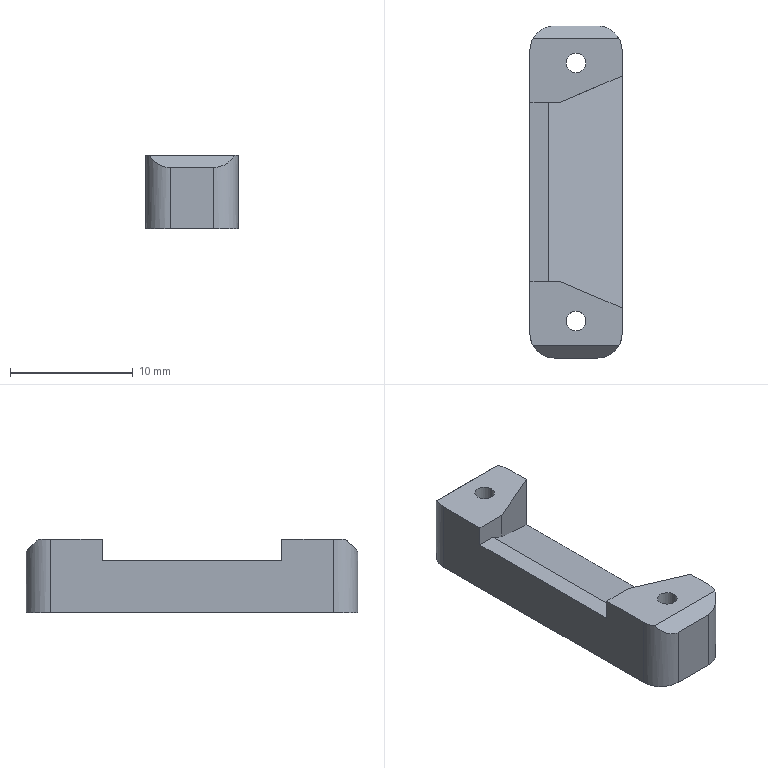NC program | NX | posted with a generic post | part box 7.5 x 27 x 6 mm
Whole program:
N10 G17 G21 G94 G90
(FLOOR_FACING , TOOL : D4-ROUGH)
N12 T01 M6
N14 G54
N16 G17 G0 G90 X20.5 Y-6. B0. C0. S4500 M3
N18 G43 Z30. H1
N20 Z2.05
N22 G94 G1 Z0.05 F800.
N24 X18.5
N26 X-25.5
N28 Y-3.15
N30 X18.5
N32 Y-0.3
N34 X-25.5
N36 Y2.55
N38 X18.5
N40 Y5.4
N42 X-25.5
N44 X-27.5
N46 Z2.05
N48 G0 Z30.
(ADAPTIVE_MILLING , TOOL : D4-ROUGH)
N50 X12.644 Y-13.007 S6500
N52 Z-4.
N54 G1 X12.632 Y-12.858 Z-4.937 F3000.
N56 X12.62 Y-12.708 Z-5.308
N58 X12.609 Y-12.558 Z-5.58
N60 X12.597 Y-12.409 Z-5.8
N62 X12.586 Y-12.259 Z-5.984
N64 X12.574 Y-12.11 Z-6.142
N66 X12.562 Y-11.96 Z-6.28
N68 X12.551 Y-11.811 Z-6.4
N70 X12.539 Y-11.661 Z-6.505
N72 X12.528 Y-11.512 Z-6.598
N74 X12.516 Y-11.362 Z-6.679
N76 X12.504 Y-11.212 Z-6.75
N78 X12.493 Y-11.063 Z-6.81
N80 X12.481 Y-10.913 Z-6.862
N82 X12.469 Y-10.764 Z-6.905
N84 X12.458 Y-10.614 Z-6.939
N86 X12.446 Y-10.465 Z-6.966
N88 X12.435 Y-10.315 Z-6.985
N90 X12.423 Y-10.166 Z-6.996
N92 X12.411 Y-10.016 Z-7.
N94 X12.385 Y-9.631
N96 X12.343 Y-9.248
N98 G3 X12.139 Y-9. R0.411
N100 X10.441 Y-8.678 R4.8
N102 X4.61 Y-8.6 R119.19
N104 G1 X-22.42 Y-8.595
N106 G2 X-24.273 Y-7.318 R2.392
N108 X-24.996 Y-4.583 R6.41
N110 X-25.098 Y0.305 R72.272
N112 G1 X-25.084 Y6.056
N114 G2 X-23.686 Y7.858 R2.494
N116 X-21.022 Y8.504 R6.789
N118 X-14.784 Y8.6 R101.69
N120 G1 X15.404 Y8.599
N122 G2 X17.251 Y7.371 R2.358
N124 X17.976 Y4.794 R6.037
N126 X18.096 Y0.027 R59.589
N128 X18.08 Y-6.087 R351.529
N130 X16.659 Y-7.873 R2.516
N132 X13.962 Y-8.508 R6.951
N134 X11.484 Y-8.375 R13.968
N136 G3 X5.808 Y-8.202 R66.934
N138 G1 X3.17 Y-8.2
N140 X-21.22 Y-8.196
N142 G2 X-23.83 Y-6.438 R3.102
N144 X-24.577 Y-3.491 R7.626
N146 X-24.697 Y1.456 R66.876
N148 X-24.67 Y5.035 R58.858
N150 X-22.813 Y7.399 R3.188
N152 X-19.762 Y8.098 R8.244
N154 X-12.864 Y8.2 R115.56
N156 G1 X14.204
N158 G2 X16.795 Y6.508 R3.064
N160 X17.574 Y3.508 R7.495
N162 X17.696 Y-1.65 R69.612
N164 X17.67 Y-5.036 R56.842
N166 X15.82 Y-7.396 R3.181
N168 X12.634 Y-7.984 R6.699
N170 G3 X2.45 Y-7.8 R183.554
N172 G1 X-20.14 Y-7.797
N174 G2 X-23.411 Y-5.696 R3.573
N176 X-24.178 Y-2.476 R8.723
N178 X-24.276 Y4.061 R79.928
N180 X-22.101 Y6.961 R3.606
N182 X-18.807 Y7.693 R9.218
N184 X-12.119 Y7.8 R111.311
N186 G1 X13.191 Y7.799
N188 G2 X16.394 Y5.733 R3.555
N190 X17.17 Y2.545 R8.578
N192 X17.27 Y-4.111 R75.06
N194 X14.894 Y-7.032 R3.582
N196 X11.737 Y-7.494 R8.667
N198 G3 X3.2 Y-7.4 R494.474
N200 G1 X-19.3 Y-7.396
N202 G2 X-23.052 Y-4.918 R3.966
N204 X-23.786 Y-1.504 R10.045
N206 X-23.855 Y3.413 R41.458
N208 X-21.509 Y6.512 R3.917
N210 X-18.161 Y7.275 R9.576
N212 X-11.653 Y7.4 R95.247
N214 G1 X12.074
N216 G2 X16.057 Y4.907 R3.995
N218 X16.789 Y1.431 R10.225
N220 X16.859 Y-3.366 R45.312
N222 X14.249 Y-6.556 R3.798
N224 X11.089 Y-7.037 R9.799
N226 G1 X1.91 Y-7.
N228 X-18.34 Y-6.997
N230 G2 X-21.223 Y-6.167 R4.515
N232 X-22.992 Y-3.299 R5.233
N234 X-23.454 Y0.715 R17.702
N236 X-23.382 Y3.109 R11.55
N238 X-20.878 Y6.107 R4.192
N240 X-17.438 Y6.871 R10.238
N242 X-10.781 Y6.999 R97.585
N244 G1 X11.204 Y7.
N246 G2 X13.836 Y6.43 R4.91
N248 X15.896 Y3.622 R4.843
N250 X16.44 Y-0.349 R15.281
N252 X16.403 Y-2.985 R14.999
N254 X13.826 Y-6.02 R3.954
N256 X10.44 Y-6.596 R10.143
N258 X1.1 Y-6.6 R586.341
N260 G1 X-17.55 Y-6.597
N262 G2 X-20.222 Y-6.046 R5.358
N264 X-22.425 Y-3.215 R4.925
N266 X-23.027 Y0.747 R14.496
N268 X-22.721 Y3.317 R5.972
N270 X-20.014 Y5.814 R4.614
N272 X-16.342 Y6.497 R12.221
N274 X-8.304 Y6.6 R157.367
N276 G1 X10.604 Y6.598
N278 G2 X13.321 Y5.992 R5.18
N280 X15.47 Y3.078 R5.03
N282 X16.036 Y-1.101 R15.78
N284 X15.417 Y-3.866 R4.67
N286 X12.628 Y-5.776 R4.734
N288 X8.972 Y-6.193 R14.778
N290 G1 X7.232 Y-6.208
N292 X-10.456 Y-6.204
N294 G2 X-17.609 Y-6.175 R433.58
N296 X-21.802 Y-3.212 R4.627
N298 X-22.523 Y1.849 R11.022
N300 X-19.878 Y5.221 R4.433
N302 X-16.182 Y6.059 R10.727
N304 X-9.99 Y6.198 R88.623
N306 G1 X9.79 Y6.2
N308 G2 X12.327 Y5.809 R6.448
N310 X14.294 Y4.819 R4.458
N312 X15.561 Y2.607 R4.476
N314 G1 X15.65 Y1.749
N316 Y-1.751
N318 X15.546 Y-2.673
N320 X15.239 Y-3.551
N322 X14.745 Y-4.337
N324 X14.087 Y-4.995
N326 X13.301 Y-5.489
N328 X12.423 Y-5.796
N330 X11.5 Y-5.9
N332 X-11.501
N334 G3 X-16.303 Y-5.797 R64.238
N336 G2 X-19.105 Y-5.259 R6.166
N338 X-21.567 Y-2.233 R5.158
N340 X-22.028 Y1.428 R8.25
N342 X-19.401 Y4.778 R4.46
N344 X-15.681 Y5.647 R10.697
N346 X-12.415 Y5.785 R72.636
N348 X-11.499 Y5.9 R3.787
N350 G1 X11.501
N352 G2 X12.347 Y5.803 R7.502
N354 G3 X12.82 Y6.348 R0.4
N356 X12.567 Y6.59 Z-6.955 R0.548
N358 G1 X12.204 Y6.819 Z-6.9
N360 X11.738 Y7.108 F15000.
N362 X11.657 Y7.132
N364 X11.574 Y7.143
N366 X-11.641 Y7.125
N368 G3 X-12.018 Y6.86 R0.401
N370 G1 X-12.076 Y6.51 Z-6.945 F3000.
N372 X-12.118 Y6.158 Z-6.99
N374 X-12.13 Y6.082 Z-7.
N376 G2 X-12.415 Y5.785 R0.402
N378 X-14.107 Y5.528 R8.134
N380 G3 X-17.929 Y5.004 R19.887
N382 X-20.854 Y3.172 R5.32
N384 X-21.679 Y-0.221 R4.872
N386 X-20.236 Y-3.903 R6.311
N388 X-17.026 Y-5.43 R4.937
N390 X-13.014 Y-5.593 R52.658
N392 X-11.738 Y-5.873 R3.505
N394 G2 X-12.984 Y-5.6 R3.404
N396 G3 X-15.088 Y-5.2 R7.056
N398 G2 X-17.861 Y-4.754 R11.202
N400 X-20.896 Y-1.405 R4.893
N402 X-20.726 Y2.106 R4.789
N404 X-17.971 Y4.394 R4.824
N406 X-14.715 Y5.048 R13.604
N408 G3 X-13.797 Y5.187 R3.561
N410 G2 X-12.705 Y5.706 R3.586
N412 G3 X-13.921 Y5.112 R3.961
N414 G2 X-15.964 Y4.648 R12.273
N416 G3 X-19.001 Y3.502 R7.713
N418 X-20.662 Y-0.761 R4.201
N420 X-17.01 Y-4.615 R4.682
N422 X-14.238 Y-5.062 R33.87
N424 G1 X-13.819 Y-5.163
N426 X-13.301 Y-5.489
N428 G3 X-14.702 Y-4.76 R4.998
N430 G2 X-17.049 Y-4.13 R32.062
N432 X-20.048 Y0.515 R4.386
N434 X-17.922 Y3.389 R3.99
N436 X-15.133 Y4.358 R11.169
N438 G3 X-14.494 Y4.595 R1.572
N440 G2 X-13.811 Y5.174 R2.943
N442 G3 X-14.619 Y4.48 R4.496
N444 G2 X-16.301 Y3.804 R9.75
N446 G3 X-18.77 Y2.262 R5.667
N448 X-18.251 Y-2.958 R3.708
N450 X-15.823 Y-4.171 R6.478
N452 G2 X-14.434 Y-4.652 R8.607
N454 G1 X-14.062 Y-5.011
N456 G3 X-15.558 Y-3.954 R3.954
N458 G2 X-17.711 Y-2.685 R7.477
N460 X-17.68 Y2.264 R3.248
N462 X-15.497 Y3.592 R8.764
N464 G3 X-14.868 Y4.175 R0.994
N466 G1 X-14.528 Y4.556
N468 G3 X-15.073 Y3.819 R2.508
N470 G2 X-16.347 Y2.914 R6.844
N472 G3 X-18.093 Y1.023 R4.263
N474 X-17.232 Y-2.462 R3.178
N476 X-15.333 Y-3.76 R9.128
N478 G2 X-14.745 Y-4.337 R1.154
N480 G1 X-14.554 Y-4.528
N482 G2 X-15.056 Y-3.851 R2.83
N484 G3 X-16.37 Y-2.657 R17.482
N486 G2 X-17.465 Y-0.223 R3.065
N488 X-16.238 Y2.159 R3.813
N490 G3 X-15.462 Y2.933 R10.353
N492 G2 X-15.042 Y3.87 R2.877
N494 G3 X-15.47 Y2.891 R2.808
N496 G2 X-16.393 Y1.601 R24.073
N498 G3 X-16.319 Y-1.968 R3.072
N500 X-15.381 Y-3.147 R40.477
N502 X-15.016 Y-3.906 R2.112
N504 G2 X-15.487 Y-2.842 R3.397
N506 X-16.157 Y-1.237 R8.879
N508 X-15.74 Y1.378 R4.04
N510 G3 X-15.65 Y1.751 R0.765
N512 G1 X-15.561 Y2.607
N514 X-15.459 Y2.921
N516 X-15.561 Y2.607
N518 G2 X-15.861 Y0.299 R19.895
N520 G3 X-15.65 Y-1.585 R5.096
N522 G1 X-15.546 Y-2.673
N524 X-15.487 Y-2.843
N526 X-15.546 Y-2.673
N528 X-15.65 Y-1.585
N530 Y1.595
N532 G3 X-16.032 Y1.998 R0.404
N534 G1 X-16.608 Y2.03
N536 X-16.758 Y2.038 Z-6.996
N538 X-16.908 Y2.046 Z-6.985
N540 X-17.058 Y2.054 Z-6.966
N542 X-17.208 Y2.063 Z-6.939
N544 X-17.357 Y2.071 Z-6.905
N546 X-17.507 Y2.079 Z-6.862
N548 X-17.657 Y2.087 Z-6.81
N550 X-17.807 Y2.095 Z-6.75
N552 X-17.956 Y2.103 Z-6.679
N554 X-18.106 Y2.112 Z-6.598
N556 X-18.256 Y2.12 Z-6.505
N558 X-18.406 Y2.128 Z-6.4
N560 X-18.556 Y2.136 Z-6.28
N562 X-18.705 Y2.144 Z-6.142
N564 X-18.855 Y2.152 Z-5.984
N566 X-19.005 Y2.16 Z-5.8
N568 X-19.155 Y2.169 Z-5.58
N570 X-19.304 Y2.177 Z-5.308
N572 X-19.454 Y2.185 Z-4.937
N574 X-19.604 Y2.193 Z-4.
N576 G0 Z30.
N578 X-9.298 Y9.877
N580 Z-1.
N582 G1 X-9.307 Y9.728 Z-1.937
N584 X-9.315 Y9.578 Z-2.308
N586 X-9.324 Y9.428 Z-2.58
N588 X-9.332 Y9.278 Z-2.8
N590 X-9.341 Y9.129 Z-2.984
N592 X-9.349 Y8.979 Z-3.142
N594 X-9.358 Y8.829 Z-3.28
N596 X-9.366 Y8.679 Z-3.4
N598 X-9.375 Y8.53 Z-3.505
N600 X-9.383 Y8.38 Z-3.598
N602 X-9.392 Y8.23 Z-3.679
N604 X-9.4 Y8.08 Z-3.75
N606 X-9.409 Y7.93 Z-3.81
N608 X-9.417 Y7.781 Z-3.862
N610 X-9.426 Y7.631 Z-3.905
N612 X-9.434 Y7.481 Z-3.939
N614 X-9.443 Y7.331 Z-3.966
N616 X-9.452 Y7.182 Z-3.985
N618 X-9.46 Y7.032 Z-3.996
N620 X-9.469 Y6.882 Z-4.
N622 X-9.492 Y6.54
N624 X-9.498 Y6.197
N626 G3 X-9.156 Y5.859 R0.405
N628 G1 X-8.008 Y5.641
N630 G3 X-3.597 Y5.503 R43.596
N632 G1 X8.139 Y5.5
N634 X8.278 Y5.555
N636 G3 X8.426 Y5.882 R0.404
N638 G1 X8.346 Y6.664 Z-3.9
N640 X8.302 Y7.06 F15000.
N642 X8.274 Y7.458
N644 G2 X9.047 Y7.559 R0.4
N646 G1 X9.295 Y6.886
N648 X9.494 Y6.331 Z-3.975 F3000.
N650 X9.498 Y6.233 Z-3.988
N652 X9.483 Y6.137 Z-4.
N654 G2 X9.157 Y5.859 R0.402
N656 G3 X8.172 Y5.49 R2.183
N658 G2 X6.193 Y5.284 R7.868
N660 X-6.531 Y5.307 R461.951
N662 X-8.165 Y5.478 R8.722
N664 G1 X-8.218 Y5.507
N666 G2 X-8.388 Y5.912 R0.463
N668 G1 X-8.418 Y6.698 Z-3.9
N670 X-8.426 Y6.865 F15000.
N672 X-8.409 Y7.033
N674 G2 X-7.76 Y7.215 R0.4
N676 G1 X-7.545 Y7.015
N678 G2 X-7.729 Y6.389 R0.4
N680 X-8.085 Y6.417 Z-3.946 R0.536 F3000.
N682 G1 X-8.487 Y6.539 Z-4.
N684 G3 X-9.053 Y6.32 R0.419
N686 X-8.843 Y5.815 R0.4
N688 G2 X-7.99 Y5.35 R3.523
N690 G3 X-6.785 Y5.037 R4.455
N692 G1 X7.259 Y5.041
N694 G3 X7.842 Y5.182 R1.055
N696 G1 X8.276 Y5.552
N698 G2 X7.607 Y5.053 R2.385
N700 G1 X7.186 Y5.037
N702 G2 X6.84 Y5.237 R0.402
N704 G1 X6.765 Y5.367
N706 X6.401 Y5.986 Z-3.908
N708 X6.354 Y6.034 Z-3.9
N710 G3 X6.092 Y6.131 R0.413 F15000.
N712 G1 X-5.691
N714 G3 X-5.938 Y6.046 R0.416
N716 G1 X-6.047 Y5.917 Z-3.922 F3000.
N718 X-6.131 Y5.77 Z-3.943
N720 X-6.355 Y5.383 Z-4.
N722 X-6.431 Y5.25
N724 X-6.528 Y5.131
N726 G2 X-6.785 Y5.037 R0.413
N728 X-7.824 Y5.17 R2.228
N730 G1 X-8.168 Y5.461
N732 G3 X-7.576 Y5.047 R1.555
N734 G1 X-7.186 Y5.037
N736 G3 X-6.783 Y5.419 R0.404
N738 G1 X-6.749 Y6.029
N740 X-6.741 Y6.179 Z-3.996
N742 X-6.733 Y6.329 Z-3.985
N744 X-6.725 Y6.479 Z-3.966
N746 X-6.716 Y6.628 Z-3.939
N748 X-6.708 Y6.778 Z-3.905
N750 X-6.7 Y6.928 Z-3.862
N752 X-6.692 Y7.078 Z-3.81
N754 X-6.683 Y7.227 Z-3.75
N756 X-6.675 Y7.377 Z-3.679
N758 X-6.667 Y7.527 Z-3.598
N760 X-6.659 Y7.677 Z-3.505
N762 X-6.65 Y7.827 Z-3.4
N764 X-6.642 Y7.976 Z-3.28
N766 X-6.634 Y8.126 Z-3.142
N768 X-6.626 Y8.276 Z-2.984
N770 X-6.618 Y8.426 Z-2.8
N772 X-6.609 Y8.575 Z-2.58
N774 X-6.601 Y8.725 Z-2.308
N776 X-6.593 Y8.875 Z-1.937
N778 X-6.585 Y9.025 Z-1.
N780 G0 Z30.
N782 X-5.37 Y8.304
N784 Z0.
N786 G1 X-5.472 Y8.193 Z-0.937
N788 X-5.573 Y8.083 Z-1.308
N790 X-5.674 Y7.972 Z-1.58
N792 X-5.776 Y7.862 Z-1.8
N794 X-5.877 Y7.751 Z-1.984
N796 X-5.978 Y7.641 Z-2.142
N798 X-6.08 Y7.53 Z-2.28
N800 X-6.181 Y7.419 Z-2.4
N802 X-6.283 Y7.309 Z-2.505
N804 X-6.384 Y7.198 Z-2.598
N806 X-6.485 Y7.088 Z-2.679
N808 X-6.587 Y6.977 Z-2.75
N810 X-6.688 Y6.867 Z-2.81
N812 X-6.789 Y6.756 Z-2.862
N814 X-6.891 Y6.645 Z-2.905
N816 X-6.992 Y6.535 Z-2.939
N818 X-7.094 Y6.424 Z-2.966
N820 X-7.195 Y6.314 Z-2.985
N822 X-7.296 Y6.203 Z-2.996
N824 X-7.398 Y6.093 Z-3.
N826 X-7.751 Y5.708
N828 G3 X-7.613 Y5.063 R0.404
N830 X-5.788 Y4.73 R5.16
N832 X-0.126 Y4.651 R134.513
N834 X6.927 Y4.657 R526.816
N836 X7.626 Y4.87 R1.103
N838 G1 X7.788 Y5.12
N840 G2 X7.032 Y4.572 R0.916
N842 X4.298 Y4.411 R15.931
N844 X-5.295 Y4.475 R289.605
N846 X-7.546 Y4.854 R6.898
N848 G1 X-7.706 Y4.987
N850 G2 X-7.771 Y5.248 R0.414
N852 G1 X-7.743 Y5.541
N854 X-7.666 Y6.323 Z-2.9
N856 X-7.65 Y6.479 F15000.
N858 X-7.657 Y6.636
N860 G3 X-7.876 Y6.987 R0.829
N862 X-8.518 Y6.753 R0.4
N864 X-8.433 Y6.395 Z-2.948 R0.52 F3000.
N866 G1 X-8.249 Y6.031 Z-3.
N868 X-7.802 Y5.145
N870 G3 X-6.908 Y4.456 R1.367
N872 X-3.94 Y4.063 R11.031
N874 X5.743 Y4.062 R174.984
N876 X7.308 Y4.392 R3.968
N878 X7.64 Y4.879 R1.907
N880 G2 X7.293 Y4.348 R2.197
N882 X5.752 Y3.887 R3.265
N884 X0.894 Y3.77 R52.587
N886 X-5.048 Y3.904 R78.332
N888 X-7.252 Y4.435 R5.835
N890 X-7.664 Y4.918 R1.036
N892 G3 X-6.409 Y3.883 R1.875
N894 X-3.383 Y3.443 R11.566
N896 X5.062 Y3.454 R100.947
N898 X7.032 Y3.909 R5.095
N900 X7.266 Y4.128 R0.677
N902 G1 X7.443 Y4.542
N904 G2 X7.122 Y3.923 R1.767
N906 X5.554 Y3.331 R3.178
N908 X1.75 Y3.138 R28.078
N910 X-4.46 Y3.295 R67.276
N912 X-6.869 Y3.9 R6.621
N914 X-7.458 Y4.576 R1.005
N916 G3 X-6.344 Y3.436 R1.737
N918 X-3.851 Y2.893 R8.511
N920 X4.853 Y2.911 R424.98
N922 X6.942 Y3.502 R4.396
N924 X7.247 Y4.083 R1.663
N926 G2 X6.875 Y3.402 R1.739
N928 X5.751 Y2.893 R2.72
N930 G1 X4.551
N932 G3 X6.256 Y2.915 R18.776
N934 X6.899 Y3.272 R0.894
N936 G1 X7.041 Y3.603
N938 G2 X6.687 Y3.019 R1.162
N940 X6.063 Y2.893 R0.881
N942 G3 X6.683 Y2.974 R1.088
N944 X6.877 Y3.22 R0.992
N946 X6.823 Y3.624 R0.402
N948 X6.489 Y3.791 Z-2.951 R0.513
N950 G1 X6.096 Y3.879 Z-2.9
N952 X5.818 Y3.943 F15000.
N954 X5.537 Y3.993
N956 X-2.813 Y3.983
N958 X-2.921 Y3.95
N960 X-3.017 Y3.891
N962 X-3.118 Y3.763 Z-2.921 F3000.
N964 X-3.198 Y3.621 Z-2.941
N966 X-3.429 Y3.224 Z-3.
N968 X-3.5 Y3.097
N970 X-3.594 Y2.986
N972 G2 X-3.851 Y2.893 R0.413
N974 X-6.161 Y3.184 R5.978
N976 X-7.132 Y3.815 R2.022
N978 G1 X-7.285 Y4.174
N980 G3 X-5.961 Y2.893 R1.838
N982 G1 X-4.701
N984 X-6.134 Y2.905
N986 G2 X-6.947 Y3.385 R1.314
N988 G1 X-7.077 Y3.688
N990 G3 X-6.596 Y2.952 R1.411
N992 X-6.021 Y2.893 R1.247
N994 G2 X-6.678 Y2.976 R1.224
N996 X-6.9 Y3.275 R0.705
N998 G3 X-6.683 Y2.974 R0.613
N1000 G1 X-6.628 Y2.949
N1002 G3 X-6.055 Y3.272 R0.404
N1004 G1 X-5.991 Y3.875
N1006 X-5.974 Y4.024 Z-2.996
N1008 X-5.958 Y4.173 Z-2.985
N1010 X-5.942 Y4.323 Z-2.966
N1012 X-5.926 Y4.472 Z-2.939
N1014 X-5.91 Y4.621 Z-2.905
N1016 X-5.894 Y4.77 Z-2.862
N1018 X-5.878 Y4.919 Z-2.81
N1020 X-5.862 Y5.068 Z-2.75
N1022 X-5.846 Y5.217 Z-2.679
N1024 X-5.83 Y5.367 Z-2.598
N1026 X-5.814 Y5.516 Z-2.505
N1028 X-5.798 Y5.665 Z-2.4
N1030 X-5.782 Y5.814 Z-2.28
N1032 X-5.766 Y5.963 Z-2.142
N1034 X-5.75 Y6.112 Z-1.984
N1036 X-5.734 Y6.261 Z-1.8
N1038 X-5.718 Y6.41 Z-1.58
N1040 X-5.702 Y6.56 Z-1.308
N1042 X-5.686 Y6.709 Z-0.937
N1044 X-5.67 Y6.858 Z0.
N1046 G0 Z30.
N1048 X-4.118 Y6.226
N1050 Z1.
N1052 G1 X-4.22 Y6.116 Z0.063
N1054 X-4.322 Y6.006 Z-0.308
N1056 X-4.423 Y5.895 Z-0.58
N1058 X-4.525 Y5.785 Z-0.8
N1060 X-4.626 Y5.674 Z-0.984
N1062 X-4.728 Y5.564 Z-1.142
N1064 X-4.83 Y5.454 Z-1.28
N1066 X-4.931 Y5.343 Z-1.4
N1068 X-5.033 Y5.233 Z-1.505
N1070 X-5.134 Y5.123 Z-1.598
N1072 X-5.236 Y5.012 Z-1.679
N1074 X-5.338 Y4.902 Z-1.75
N1076 X-5.439 Y4.792 Z-1.81
N1078 X-5.541 Y4.681 Z-1.862
N1080 X-5.642 Y4.571 Z-1.905
N1082 X-5.744 Y4.461 Z-1.939
N1084 X-5.846 Y4.35 Z-1.966
N1086 X-5.947 Y4.24 Z-1.985
N1088 X-6.049 Y4.13 Z-1.996
N1090 X-6.151 Y4.019 Z-2.
N1092 X-6.583 Y3.55
N1094 G3 X-6.462 Y2.912 R0.404
N1096 X-4.739 Y2.571 R4.565
N1098 X1.03 Y2.493 R116.156
N1100 X5.898 Y2.52 R120.49
N1102 X6.655 Y2.764 R1.304
N1104 G1 X6.794 Y3.028
N1106 G2 X6.134 Y2.465 R0.804
N1108 X3.819 Y2.269 R10.582
N1110 X-4.39 Y2.324 R166.147
N1112 X-6.595 Y2.769 R6.073
N1114 G1 X-6.758 Y2.942
N1116 G2 X-6.612 Y3.43 R0.401
N1118 X-6.187 Y3.451 Z-1.943 R0.437
N1120 G1 X-5.866 Y3.34 Z-1.9
N1122 G3 X-5.53 Y3.274 R0.681 F15000.
N1124 X-5.226 Y3.826 R0.4
N1126 X-5.617 Y4.148 R0.437
N1128 X-5.861 Y4.074 R0.418
N1130 G1 X-6.082 Y3.915
N1132 X-6.404 Y3.69 Z-1.95 F3000.
N1134 X-6.717 Y3.452 Z-2.
N1136 G3 X-6.792 Y3.022 R0.402
N1138 X-6.117 Y2.407 R1.078
N1140 X-3.609 Y1.938 R7.557
N1142 X4.815 Y1.923 R104.184
N1144 X6.435 Y2.328 R3.58
N1146 X6.711 Y2.833 R1.326
N1148 G2 X6.409 Y2.271 R1.449
N1150 X4.846 Y1.753 R3.096
N1152 X0.225 Y1.618 R43.911
N1154 X-4.616 Y1.819 R38.528
N1156 X-6.49 Y2.461 R4.083
N1158 X-6.723 Y2.86 R0.921
N1160 G3 X-5.705 Y1.844 R1.571
N1162 X-2.939 Y1.317 R8.88
N1164 X4.328 Y1.332 R58.831
N1166 X6.228 Y1.863 R4.361
N1168 X6.54 Y2.435 R1.4
N1170 G2 X6.219 Y1.815 R1.803
N1172 X4.617 Y1.192 R3.226
N1174 X0.491 Y0.991 R27.661
N1176 X-4.276 Y1.25 R30.921
N1178 X-6.261 Y1.992 R4.461
N1180 X-6.572 Y2.509 R1.082
N1182 G3 X-5.415 Y1.301 R1.823
N1184 X-2.983 Y0.748 R8.271
N1186 X3.854 Y0.764 R512.921
N1188 X6.02 Y1.373 R4.594
N1190 X6.341 Y1.97 R1.528
N1192 G2 X6.012 Y1.323 R2.042
N1194 X4.801 Y0.748 R2.672
N1196 G1 X3.601
N1198 G3 X5.316 Y0.772 R16.877
N1200 X5.985 Y1.139 R0.939
N1202 G1 X6.138 Y1.497
N1204 G2 X5.838 Y0.936 R1.46
N1206 X5.126 Y0.748 R0.884
N1208 G3 X5.764 Y0.83 R1.135
N1210 X5.969 Y1.103 R0.839
N1212 X5.916 Y1.508 R0.402
N1214 X5.581 Y1.675 Z-1.951 R0.513
N1216 G1 X5.189 Y1.762 Z-1.9
N1218 X4.911 Y1.827 F15000.
N1220 X4.629 Y1.876
N1222 X-1.945 Y1.838
N1224 X-2.052 Y1.805
N1226 X-2.147 Y1.746
N1228 X-2.249 Y1.619 Z-1.921 F3000.
N1230 X-2.329 Y1.478 Z-1.941
N1232 X-2.56 Y1.08 Z-2.
N1234 X-2.633 Y0.953
N1236 X-2.727 Y0.841
N1238 G2 X-2.983 Y0.748 R0.413
N1240 X-5.478 Y1.152 R5.451
N1242 X-6.224 Y1.697 R1.813
N1244 G1 X-6.378 Y2.056
N1246 G3 X-5.792 Y1.144 R1.883
N1248 X-5.024 Y0.748 R2.16
N1250 G1 X-3.764
N1252 G2 X-5.264 Y0.775 R11.399
N1254 X-6.035 Y1.256 R1.326
N1256 G1 X-6.177 Y1.587
N1258 G3 X-5.697 Y0.824 R1.556
N1260 X-5.072 Y0.748 R1.155
N1262 G2 X-5.759 Y0.831 R1.298
N1264 X-5.993 Y1.158 R0.716
N1266 G3 X-5.764 Y0.83 R0.655
N1268 G1 X-5.676 Y0.789
N1270 X-5.584 Y0.762
N1272 G3 X-5.122 Y1.166 R0.404
N1274 G1 X-5.127 Y1.731
N1276 X-5.129 Y1.881 Z-1.996
N1278 X-5.13 Y2.031 Z-1.985
N1280 X-5.131 Y2.181 Z-1.966
N1282 X-5.133 Y2.331 Z-1.939
N1284 X-5.134 Y2.481 Z-1.905
N1286 X-5.136 Y2.631 Z-1.862
N1288 X-5.137 Y2.781 Z-1.81
N1290 X-5.139 Y2.931 Z-1.75
N1292 X-5.14 Y3.081 Z-1.679
N1294 X-5.141 Y3.231 Z-1.598
N1296 X-5.143 Y3.381 Z-1.505
N1298 X-5.144 Y3.531 Z-1.4
N1300 X-5.146 Y3.681 Z-1.28
N1302 X-5.147 Y3.831 Z-1.142
N1304 X-5.149 Y3.981 Z-0.984
N1306 X-5.15 Y4.13 Z-0.8
N1308 X-5.152 Y4.28 Z-0.58
N1310 X-5.153 Y4.43 Z-0.308
N1312 X-5.154 Y4.58 Z0.063
N1314 X-5.156 Y4.73 Z1.
N1316 G0 Z30.
N1318 X7.925 Y-9.851
N1320 Z1.451
N1322 G1 X7.904 Y-9.702 Z0.514
N1324 X7.882 Y-9.554 Z0.143
N1326 X7.86 Y-9.405 Z-0.129
N1328 X7.839 Y-9.257 Z-0.349
N1330 X7.817 Y-9.108 Z-0.533
N1332 X7.795 Y-8.96 Z-0.691
N1334 X7.774 Y-8.812 Z-0.829
N1336 X7.752 Y-8.663 Z-0.949
N1338 X7.73 Y-8.515 Z-1.054
N1340 X7.708 Y-8.366 Z-1.147
N1342 X7.687 Y-8.218 Z-1.228
N1344 X7.665 Y-8.07 Z-1.299
N1346 X7.643 Y-7.921 Z-1.359
N1348 X7.622 Y-7.773 Z-1.411
N1350 X7.6 Y-7.624 Z-1.454
N1352 X7.578 Y-7.476 Z-1.488
N1354 X7.556 Y-7.327 Z-1.515
N1356 X7.535 Y-7.179 Z-1.534
N1358 X7.513 Y-7.031 Z-1.545
N1360 X7.491 Y-6.882 Z-1.549
N1362 X7.392 Y-6.202
N1364 G3 X7.055 Y-5.861 R0.405
N1366 X5.388 Y-5.593 R19.887
N1368 X-0.844 Y-5.5 R103.844
N1370 G1 X-6.044 Y-5.505
N1372 X-6.636 Y-5.795
N1374 X-7.08 Y-5.865
N1376 G3 X-6.107 Y-5.525 R2.032
N1378 G2 X-4.573 Y-5.301 R4.591
N1380 X4.928 Y-5.337 R158.736
N1382 X6.038 Y-5.49 R4.054
N1384 G1 X6.636 Y-5.795
N1386 X5.645 Y-5.27
N1388 G3 X3.053 Y-4.911 R9.22
N1390 X-4.767 Y-4.938 R100.023
N1392 X-5.657 Y-5.116 R2.19
N1394 G1 X-6.063 Y-5.503
N1396 G2 X-5.508 Y-5.012 R3.526
N1398 X-3.566 Y-4.677 R5.666
N1400 X4.007 Y-4.748 R72.432
N1402 X5.664 Y-5.123 R4.82
N1404 G1 X6.03 Y-5.483
N1406 G3 X5.134 Y-4.763 R2.715
N1408 X2.568 Y-4.307 R8.201
N1410 X-3.96 Y-4.335 R53.833
N1412 X-5.338 Y-4.669 R3.794
N1414 X-5.561 Y-5.014 R1.168
N1416 G1 X-5.645 Y-5.099
N1418 G3 X-5.404 Y-4.712 R1.224
N1420 G2 X-4.253 Y-4.218 R2.156
N1422 X-0.483 Y-3.999 R21.812
N1424 X3.946 Y-4.24 R28.092
N1426 X5.402 Y-4.752 R3.618
N1428 G1 X5.561 Y-5.014
N1430 G3 X4.629 Y-4.186 R1.474
N1432 X1.871 Y-3.684 R9.202
N1434 X-3.636 Y-3.764 R31.656
N1436 X-5.158 Y-4.258 R3.374
N1438 G1 X-5.254 Y-4.408
N1440 G3 X-5.153 Y-4.74 R0.405
N1442 G1 X-4.612 Y-5.31 Z-1.449
N1444 X-4.362 Y-5.566 F15000.
N1446 G3 X-3.723 Y-5.292 R0.4
N1448 X-3.812 Y-4.883 R0.47
N1450 X-4.362 Y-4.84 R0.4
N1452 G1 X-4.856 Y-5.261 Z-1.532 F3000.
N1454 X-4.982 Y-5.311 Z-1.549
N1456 G2 X-5.42 Y-4.738 R0.4
N1458 X-5.131 Y-4.197 R2.757
N1460 X-3.602 Y-3.588 R3.078
N1462 X1.353 Y-3.428 R24.985
N1464 X4.416 Y-3.915 R10.837
N1466 X5.261 Y-4.426 R1.876
N1468 G1 X5.424 Y-4.746
N1470 G3 X4.262 Y-3.625 R1.837
N1472 X1.216 Y-3.061 R9.843
N1474 X-3.549 Y-3.231 R20.64
N1476 X-5.11 Y-3.903 R3.104
N1478 X-5.255 Y-4.414 R0.937
N1480 G2 X-5.058 Y-3.796 R1.053
N1482 X-3.763 Y-3.109 R2.907
N1484 G3 X-3.367 Y-1.226 R1.574
N1486 X-4.694 Y0.027 R2.642
N1488 G2 X-5.735 Y0.61 R5.542
N1490 G1 X-5.881 Y0.896
N1492 G3 X-5.296 Y0.1 R1.816
N1494 G2 X-4.93 Y-1.81 R2.277
N1496 G1 X-5.15 Y-2.662
N1498 G2 X-5.197 Y-4.047 R7.187
N1500 G3 X-5.15 Y-2.662 R7.187
N1502 X-5.194 Y-0.818 R14.276
N1504 X-5.761 Y0.616 R9.845
N1506 G2 X-5.194 Y-0.818 R9.845
N1508 X-5.15 Y-2.394 R12.013
N1510 G3 X-4.933 Y-2.773 R0.442
N1512 G1 X-4.761 Y-2.835 Z-1.526
N1514 X-4.581 Y-2.872 Z-1.502
N1516 X-4.173 Y-2.962 Z-1.449
N1518 X4.364 Y-4.834 F15000.
N1520 X4.595 Y-4.887 Z-1.479 F3000.
N1522 X4.829 Y-4.922 Z-1.509
N1524 G3 X5.113 Y-4.812 Z-1.549 R0.448
N1526 X5.255 Y-4.414 R0.443
N1528 X4.579 Y-3.564 R1.298
N1530 X3.314 Y-3.062 R3.306
N1532 X3.072 Y-3.138 R2.68
N1534 X3.006 Y-3.821 Z-1.449 R0.441
N1536 G1 X3.045 Y-3.855 F15000.
N1538 X3.089 Y-3.884
N1540 X4.283 Y-4.595
N1542 X4.647 Y-4.804 Z-1.503 F3000.
N1544 G3 X5.002 Y-4.788 Z-1.549 R0.454
N1546 X5.241 Y-4.325 R0.441
N1548 X4.52 Y-3.299 R1.429
N1550 G2 X3.959 Y-2.372 R0.991
N1552 X4.657 Y-0.767 R2.22
N1554 G1 X5.516 Y0.057
N1556 X5.878 Y0.89
N1558 G2 X5.14 Y-0.542 R5.663
N1560 G3 X5.045 Y-2.736 R2.982
N1562 G2 X5.15 Y-3.749 R2.462
N1564 G1 X5.216 Y-4.164
N1566 G2 X5.15 Y-3.139 R3.85
N1568 G1 Y-1.249
N1570 G2 X5.513 Y0.039 R2.994
N1572 G3 X5.292 Y0.573 R0.404
N1574 G1 X4.764 Y0.784
N1576 X4.624 Y0.839 Z-1.545
N1578 X4.485 Y0.895 Z-1.534
N1580 X4.346 Y0.95 Z-1.515
N1582 X4.206 Y1.006 Z-1.488
N1584 X4.067 Y1.062 Z-1.454
N1586 X3.928 Y1.117 Z-1.411
N1588 X3.788 Y1.173 Z-1.359
N1590 X3.649 Y1.228 Z-1.299
N1592 X3.51 Y1.284 Z-1.228
N1594 X3.37 Y1.339 Z-1.147
N1596 X3.231 Y1.395 Z-1.054
N1598 X3.092 Y1.45 Z-0.949
N1600 X2.953 Y1.506 Z-0.829
N1602 X2.813 Y1.562 Z-0.691
N1604 X2.674 Y1.617 Z-0.533
N1606 X2.535 Y1.673 Z-0.349
N1608 X2.395 Y1.728 Z-0.129
N1610 X2.256 Y1.784 Z0.143
N1612 X2.117 Y1.839 Z0.514
N1614 X1.977 Y1.895 Z1.451
N1616 G0 Z30.
N1618 M5
(FLOOR_FACING_COPY , TOOL : D4-FINISH)
N1620 T02 M6
N1622 G54
N1624 G17 G0 G90 X20.5 Y-6. B0. C0. S4500 M3
N1626 G43 Z30. H2
N1628 Z2.
N1630 G94 G1 Z0. F800.
N1632 X18.5
N1634 X-25.5
N1636 Y-3.15
N1638 X18.5
N1640 Y-0.3
N1642 X-25.5
N1644 Y2.55
N1646 X18.5
N1648 Y5.4
N1650 X-25.5
N1652 X-27.5
N1654 Z2.
N1656 G0 Z30.
(PLANAR_MILL , TOOL : D4-FINISH)
N1658 X13.465 Y-7.947 S5500
N1660 Z-5.
N1662 G1 Z-7.
N1664 G41 X13.5 Y-7.75 D2
N1666 G3 X11.5 Y-5.75 R2.
N1668 G1 X-11.5
N1670 G2 X-15.5 Y-1.75 R4.
N1672 G1 Y1.75
N1674 G2 X-11.5 Y5.75 R4.
N1676 G1 X11.5
N1678 G2 X15.5 Y1.75 R4.
N1680 G1 Y-1.75
N1682 G2 X11.5 Y-5.75 R4.
N1684 G3 X9.5 Y-7.75 R2.
N1686 G40
N1688 G1 X9.535 Y-7.947
N1690 X13.465
N1692 G41 X13.5 Y-7.75
N1694 G3 X11.5 Y-5.75 R2.
N1696 G1 X-11.5
N1698 G2 X-15.5 Y-1.75 R4.
N1700 G1 Y1.75
N1702 G2 X-11.5 Y5.75 R4.
N1704 G1 X11.5
N1706 G2 X15.5 Y1.75 R4.
N1708 G1 Y-1.75
N1710 G2 X11.5 Y-5.75 R4.
N1712 G3 X9.5 Y-7.75 R2.
N1714 G40
N1716 G1 X9.535 Y-7.947
N1718 Z-5.
N1720 G0 Z30.
(FLOOR_FACING_1 , TOOL : D4-FINISH)
N1722 X-5.247 Y-7.8 S4500
N1724 Z0.3
N1726 G1 Z-1.7
N1728 Y-5.8
N1730 Y-0.2
N1732 X-2.623
N1734 Y-5.8
N1736 X0.002
N1738 Y-0.2
N1740 X2.626
N1742 Y-5.8
N1744 X5.25
N1746 Y-0.2
N1748 Y4.248
N1750 Z0.3
N1752 G0 Z30.
(PLANAR_MILL_1 , TOOL : D4-FINISH)
N1754 X-5.265 Y1.947
N1756 Z0.3
N1758 G1 Z-1.7
N1760 G41 X-5.3 Y1.75
N1762 Y-1.25
N1764 Y-3.75
N1766 Y-6.75
N1768 G40
N1770 X-5.265 Y-6.947
N1772 Z0.3
N1774 G0 Z30.
N1776 X5.265
N1778 Z0.3
N1780 G1 Z-1.7
N1782 G41 X5.3 Y-6.75
N1784 Y-3.75
N1786 Y-1.25
N1788 Y1.75
N1790 G40
N1792 X5.265 Y1.947
N1794 Z0.3
N1796 G0 Z30.
N1798 M5
(DRILLING , TOOL : D3点钻)
N1800 T03 M6
N1802 G54
N1804 G17 G0 G90 X-10.5 Y0. B0. C0. S3000 M3
N1806 G43 Z30. H3
N1808 G94 G81 G98 Z-1. F200. R3.
N1810 X10.5
N1812 G80
N1814 G0 X10.5 Y0. Z30.
(PLANAR_MILL_2 , TOOL : D3点钻)
N1816 X12.5 Y-6.2 S3500
N1818 Z0.8
N1820 G1 Z-1.2 F800.
N1822 G3 X11.5 Y-5.2 R1.
N1824 G1 X7.3
N1826 G2 X5.85 Y-3.75 R1.45
N1828 G1 Y-1.25
N1830 G2 X5.967 Y-0.679 R1.45
N1832 G1 X8.11 Y4.321
N1834 G2 X9.443 Y5.2 R1.45
N1836 G1 X11.5
N1838 G2 X13.225 Y4.738 R3.45
N1840 X13.95 Y3.482 R1.45
N1842 G1 Y-3.482
N1844 G2 X13.225 Y-4.738 R1.45
N1846 X11.5 Y-5.2 R3.45
N1848 G3 X10.5 Y-6.2 R1.
N1850 G1 X12.5 Y-6.
N1852 G3 X11.5 Y-5. R1.
N1854 G1 X7.3
N1856 G2 X6.05 Y-3.75 R1.25
N1858 G1 Y-1.25
N1860 G2 X6.151 Y-0.758 R1.25
N1862 G1 X8.294 Y4.242
N1864 G2 X9.443 Y5. R1.25
N1866 G1 X11.5
N1868 G2 X13.125 Y4.565 R3.25
N1870 X13.75 Y3.482 R1.25
N1872 G1 Y-3.482
N1874 G2 X13.125 Y-4.565 R1.25
N1876 X11.5 Y-5. R3.25
N1878 G3 X10.5 Y-6. R1.
N1880 G1 Y-6.2
N1882 Z0.8
N1884 G0 Z30.
N1886 X-4.85 Y-2.75
N1888 Z0.8
N1890 G1 Z-1.2
N1892 G3 X-5.85 Y-3.75 R1.
N1894 G2 X-7.3 Y-5.2 R1.45
N1896 G1 X-11.5
N1898 G2 X-13.225 Y-4.738 R3.45
N1900 X-13.95 Y-3.482 R1.45
N1902 G1 Y3.482
N1904 G2 X-13.225 Y4.738 R1.45
N1906 X-11.5 Y5.2 R3.45
N1908 G1 X-9.443
N1910 G2 X-8.11 Y4.321 R1.45
N1912 G1 X-5.967 Y-0.679
N1914 G2 X-5.85 Y-1.25 R1.45
N1916 G1 Y-3.75
N1918 G3 X-4.85 Y-4.75 R1.
N1920 G1 X-5.05 Y-2.75
N1922 G3 X-6.05 Y-3.75 R1.
N1924 G2 X-7.3 Y-5. R1.25
N1926 G1 X-11.5
N1928 G2 X-13.125 Y-4.565 R3.25
N1930 X-13.75 Y-3.482 R1.25
N1932 G1 Y3.482
N1934 G2 X-13.125 Y4.565 R1.25
N1936 X-11.5 Y5. R3.25
N1938 G1 X-9.443
N1940 G2 X-8.294 Y4.242 R1.25
N1942 G1 X-6.151 Y-0.758
N1944 G2 X-6.05 Y-1.25 R1.25
N1946 G1 Y-3.75
N1948 G3 X-5.05 Y-4.75 R1.
N1950 G1 Z0.8
N1952 G0 Z30.
(PLANAR_MILL_3 , TOOL : D3点钻)
N1954 X5.765 Y-5.447
N1956 Z-0.7
N1958 G1 Z-2.7
N1960 G41 X5.8 Y-5.25 D3
N1962 G3 X5.3 Y-4.75 R0.5
N1964 G1 X-5.3
N1966 G3 X-5.8 Y-5.25 R0.5
N1968 G40
N1970 G1 X-5.765 Y-5.447
N1972 Z-0.7
N1974 G0 Z30.
N1976 M5
(DRILLING_COPY , TOOL : D1.8钻头)
N1978 T04 M6
N1980 G54
N1982 G17 G0 G90 X-10.5 Y0. B0. C0. S3000 M3
N1984 G43 Z30. H4
N1986 G94 G83 G98 Z-8. F150. Q2. R3.
N1988 X10.5
N1990 G80
N1992 G0 X10.5 Y0. Z30.
N1994 M5
N1996 M2